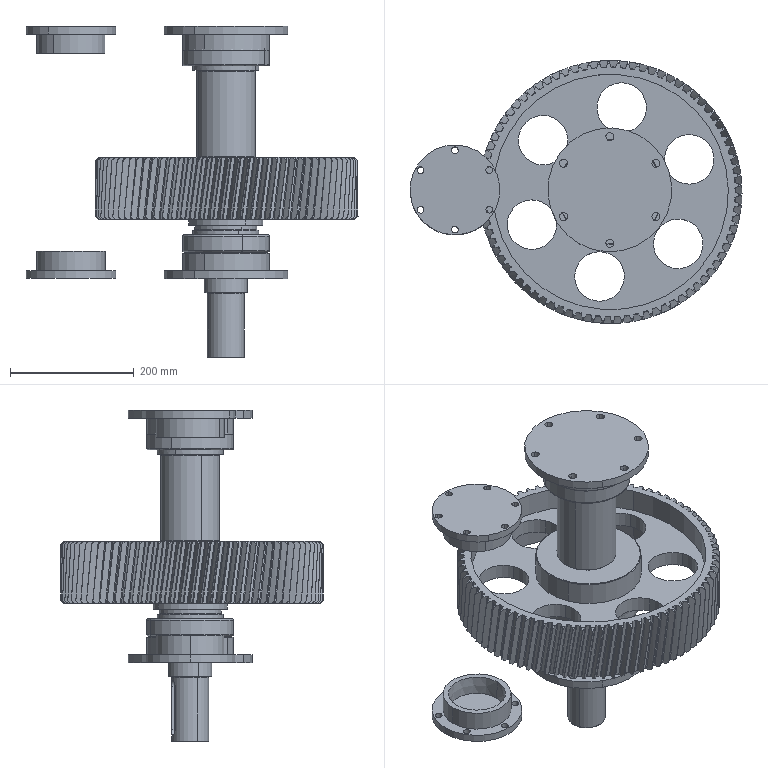Part | SolidWorks | 10 solids | 1284 faces | box 535.812 x 424.15 x 535.75 mm | volume 9344461 mm3 | spline 410 | cone 318 | cylinder 209 | torus 202 | plane 145 | commonest cylinder face diameters 424.15 x83 11 x24 13 x24 80 x22 140 x8 22 x5